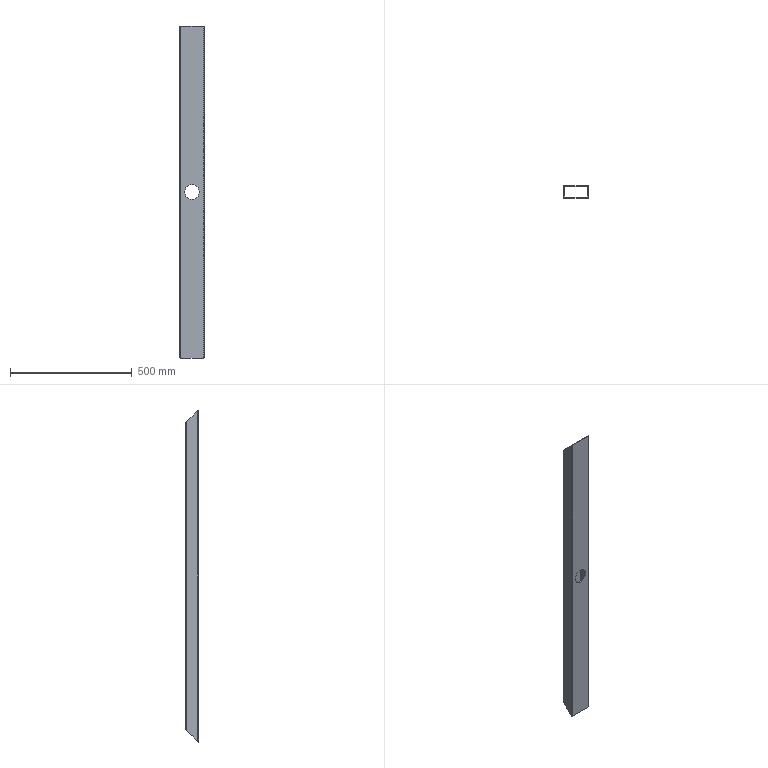Part | SolidWorks | features ICE 2, Extrusion 1 | 1 solid | 22 faces | box 100 x 50 x 1364 mm | volume 1106656 mm3 | cylinder 12 | plane 10 | commonest cylinder face diameters 0.4 x4 6.4 x4 60.3 x4
STEP:
#1=CARTESIAN_POINT('',(0.,-25.,656.26));
#2=VERTEX_POINT('',#1);
#3=CARTESIAN_POINT('',(0.,-25.,716.56));
#4=VERTEX_POINT('',#3);
#5=CARTESIAN_POINT('',(0.,-25.,686.41));
#6=DIRECTION('',(0.,1.,0.));
#7=DIRECTION('',(0.,0.,1.));
#8=AXIS2_PLACEMENT_3D('',#5,#6,#7);
#9=CIRCLE('',#8,30.15);
#10=EDGE_CURVE('',#2,#4,#9,.T.);
#11=ORIENTED_EDGE('',*,*,#10,.F.);
#12=CARTESIAN_POINT('',(0.,-22.,656.26));
#13=VERTEX_POINT('',#12);
#14=CARTESIAN_POINT('',(0.,-193.,656.26));
#15=DIRECTION('',(0.,1.,0.));
#16=VECTOR('',#15,1000.);
#17=LINE('',#14,#16);
#18=EDGE_CURVE('',#2,#13,#17,.T.);
#19=ORIENTED_EDGE('',*,*,#18,.T.);
#20=CARTESIAN_POINT('',(0.,-22.,716.56));
#21=VERTEX_POINT('',#20);
#22=CARTESIAN_POINT('',(0.,-22.,686.41));
#23=DIRECTION('',(0.,1.,0.));
#24=DIRECTION('',(0.,0.,1.));
#25=AXIS2_PLACEMENT_3D('',#22,#23,#24);
#26=CIRCLE('',#25,30.15);
#27=EDGE_CURVE('',#13,#21,#26,.T.);
#28=ORIENTED_EDGE('',*,*,#27,.T.);
#29=CARTESIAN_POINT('',(0.,-193.,716.56));
#30=DIRECTION('',(0.,1.,0.));
#31=VECTOR('',#30,1000.);
#32=LINE('',#29,#31);
#33=EDGE_CURVE('',#4,#21,#32,.T.);
#34=ORIENTED_EDGE('',*,*,#33,.F.);
#35=EDGE_LOOP('',(#11,#19,#28,#34));
#36=FACE_OUTER_BOUND('',#35,.T.);
#37=CARTESIAN_POINT('',(0.,-193.,686.41));
#38=DIRECTION('',(0.,1.,0.));
#39=DIRECTION('',(0.,0.,1.));
#40=AXIS2_PLACEMENT_3D('',#37,#38,#39);
#41=CYLINDRICAL_SURFACE('',#40,30.15);
#42=ADVANCED_FACE('',(#36),#41,.F.);
#43=CARTESIAN_POINT('',(0.,22.,716.56));
#44=VERTEX_POINT('',#43);
#45=CARTESIAN_POINT('',(0.,22.,656.26));
#46=VERTEX_POINT('',#45);
#47=CARTESIAN_POINT('',(0.,22.,686.41));
#48=DIRECTION('',(0.,-1.,0.));
#49=DIRECTION('',(0.,0.,-1.));
#50=AXIS2_PLACEMENT_3D('',#47,#48,#49);
#51=CIRCLE('',#50,30.15);
#52=EDGE_CURVE('',#44,#46,#51,.T.);
#53=ORIENTED_EDGE('',*,*,#52,.T.);
#54=CARTESIAN_POINT('',(0.,25.,656.26));
#55=VERTEX_POINT('',#54);
#56=CARTESIAN_POINT('',(0.,-193.,656.26));
#57=DIRECTION('',(0.,1.,0.));
#58=VECTOR('',#57,1000.);
#59=LINE('',#56,#58);
#60=EDGE_CURVE('',#46,#55,#59,.T.);
#61=ORIENTED_EDGE('',*,*,#60,.T.);
#62=CARTESIAN_POINT('',(0.,25.,716.56));
#63=VERTEX_POINT('',#62);
#64=CARTESIAN_POINT('',(0.,25.,686.41));
#65=DIRECTION('',(0.,1.,0.));
#66=DIRECTION('',(0.,0.,1.));
#67=AXIS2_PLACEMENT_3D('',#64,#65,#66);
#68=CIRCLE('',#67,30.15);
#69=EDGE_CURVE('',#55,#63,#68,.T.);
#70=ORIENTED_EDGE('',*,*,#69,.T.);
#71=CARTESIAN_POINT('',(0.,-193.,716.56));
#72=DIRECTION('',(0.,1.,0.));
#73=VECTOR('',#72,1000.);
#74=LINE('',#71,#73);
#75=EDGE_CURVE('',#44,#63,#74,.T.);
#76=ORIENTED_EDGE('',*,*,#75,.F.);
#77=EDGE_LOOP('',(#53,#61,#70,#76));
#78=FACE_OUTER_BOUND('',#77,.T.);
#79=CARTESIAN_POINT('',(0.,-193.,686.41));
#80=DIRECTION('',(0.,1.,0.));
#81=DIRECTION('',(0.,0.,1.));
#82=AXIS2_PLACEMENT_3D('',#79,#80,#81);
#83=CYLINDRICAL_SURFACE('',#82,30.15);
#84=ADVANCED_FACE('',(#78),#83,.F.);
#85=ORIENTED_EDGE('',*,*,#52,.F.);
#86=CARTESIAN_POINT('',(0.,22.,686.41));
#87=DIRECTION('',(0.,-1.,0.));
#88=DIRECTION('',(0.,0.,-1.));
#89=AXIS2_PLACEMENT_3D('',#86,#87,#88);
#90=CIRCLE('',#89,30.15);
#91=EDGE_CURVE('',#46,#44,#90,.T.);
#92=ORIENTED_EDGE('',*,*,#91,.F.);
#93=EDGE_LOOP('',(#85,#92));
#94=FACE_BOUND('',#93,.T.);
#95=CARTESIAN_POINT('',(-46.8,22.,1321.41));
#96=VERTEX_POINT('',#95);
#97=CARTESIAN_POINT('',(46.8,22.,1321.41));
#98=VERTEX_POINT('',#97);
#99=CARTESIAN_POINT('',(-46.8,22.,1321.41));
#100=DIRECTION('',(1.,0.,0.));
#101=VECTOR('',#100,1000.);
#102=LINE('',#99,#101);
#103=EDGE_CURVE('',#96,#98,#102,.T.);
#104=ORIENTED_EDGE('',*,*,#103,.F.);
#105=CARTESIAN_POINT('',(-46.8,22.,51.41));
#106=VERTEX_POINT('',#105);
#107=CARTESIAN_POINT('',(-46.8,22.,1400.));
#108=DIRECTION('',(0.,0.,-1.));
#109=VECTOR('',#108,1000.);
#110=LINE('',#107,#109);
#111=EDGE_CURVE('',#96,#106,#110,.T.);
#112=ORIENTED_EDGE('',*,*,#111,.T.);
#113=CARTESIAN_POINT('',(46.8,22.,51.41));
#114=VERTEX_POINT('',#113);
#115=CARTESIAN_POINT('',(-46.8,22.,51.41));
#116=DIRECTION('',(-1.,0.,0.));
#117=VECTOR('',#116,1000.);
#118=LINE('',#115,#117);
#119=EDGE_CURVE('',#114,#106,#118,.T.);
#120=ORIENTED_EDGE('',*,*,#119,.F.);
#121=CARTESIAN_POINT('',(46.8,22.,1400.));
#122=DIRECTION('',(0.,0.,-1.));
#123=VECTOR('',#122,1000.);
#124=LINE('',#121,#123);
#125=EDGE_CURVE('',#98,#114,#124,.T.);
#126=ORIENTED_EDGE('',*,*,#125,.F.);
#127=EDGE_LOOP('',(#104,#112,#120,#126));
#128=FACE_OUTER_BOUND('',#127,.T.);
#129=CARTESIAN_POINT('',(-46.8,22.,1400.));
#130=DIRECTION('',(0.,-1.,0.));
#131=DIRECTION('',(0.,0.,-1.));
#132=AXIS2_PLACEMENT_3D('',#129,#130,#131);
#133=PLANE('',#132);
#134=ADVANCED_FACE('',(#94,#128),#133,.T.);
#135=CARTESIAN_POINT('',(47.,21.8,1321.61));
#136=VERTEX_POINT('',#135);
#137=CARTESIAN_POINT('',(46.8,22.,1321.41));
#138=CARTESIAN_POINT('',(46.917,22.,1321.41));
#139=CARTESIAN_POINT('',(47.,21.917,1321.493));
#140=CARTESIAN_POINT('',(47.,21.8,1321.61));
#141=(BOUNDED_CURVE()B_SPLINE_CURVE(3,(#137,#138,#139,#140),.UNSPECIFIED.,.F.,.F.)B_SPLINE_CURVE_WITH_KNOTS((4,4),(0.,1.571),.UNSPECIFIED.)CURVE()GEOMETRIC_REPRESENTATION_ITEM()RATIONAL_B_SPLINE_CURVE((1.,0.8047,0.8047,1.))REPRESENTATION_ITEM(''));
#142=EDGE_CURVE('',#98,#136,#141,.T.);
#143=ORIENTED_EDGE('',*,*,#142,.F.);
#144=ORIENTED_EDGE('',*,*,#125,.T.);
#145=CARTESIAN_POINT('',(47.,21.8,51.21));
#146=VERTEX_POINT('',#145);
#147=CARTESIAN_POINT('',(47.,21.8,51.21));
#148=CARTESIAN_POINT('',(47.,21.917,51.327));
#149=CARTESIAN_POINT('',(46.917,22.,51.41));
#150=CARTESIAN_POINT('',(46.8,22.,51.41));
#151=(BOUNDED_CURVE()B_SPLINE_CURVE(3,(#147,#148,#149,#150),.UNSPECIFIED.,.F.,.F.)B_SPLINE_CURVE_WITH_KNOTS((4,4),(1.571,3.142),.UNSPECIFIED.)CURVE()GEOMETRIC_REPRESENTATION_ITEM()RATIONAL_B_SPLINE_CURVE((1.,0.8047,0.8047,1.))REPRESENTATION_ITEM(''));
#152=EDGE_CURVE('',#146,#114,#151,.T.);
#153=ORIENTED_EDGE('',*,*,#152,.F.);
#154=CARTESIAN_POINT('',(47.,21.8,1400.));
#155=DIRECTION('',(0.,0.,-1.));
#156=VECTOR('',#155,1000.);
#157=LINE('',#154,#156);
#158=EDGE_CURVE('',#136,#146,#157,.T.);
#159=ORIENTED_EDGE('',*,*,#158,.F.);
#160=EDGE_LOOP('',(#143,#144,#153,#159));
#161=FACE_OUTER_BOUND('',#160,.T.);
#162=CARTESIAN_POINT('',(46.8,21.8,1400.));
#163=DIRECTION('',(0.,0.,-1.));
#164=DIRECTION('',(-1.,0.,0.));
#165=AXIS2_PLACEMENT_3D('',#162,#163,#164);
#166=CYLINDRICAL_SURFACE('',#165,0.2);
#167=ADVANCED_FACE('',(#161),#166,.F.);
#168=CARTESIAN_POINT('',(47.,-21.8,1365.21));
#169=VERTEX_POINT('',#168);
#170=CARTESIAN_POINT('',(47.,-17.395,1360.805));
#171=DIRECTION('',(0.,-0.7071,0.7071));
#172=VECTOR('',#171,1000.);
#173=LINE('',#170,#172);
#174=EDGE_CURVE('',#136,#169,#173,.T.);
#175=ORIENTED_EDGE('',*,*,#174,.F.);
#176=ORIENTED_EDGE('',*,*,#158,.T.);
#177=CARTESIAN_POINT('',(47.,-21.8,7.61));
#178=VERTEX_POINT('',#177);
#179=CARTESIAN_POINT('',(47.,696.195,725.605));
#180=DIRECTION('',(0.,0.7071,0.7071));
#181=VECTOR('',#180,1000.);
#182=LINE('',#179,#181);
#183=EDGE_CURVE('',#178,#146,#182,.T.);
#184=ORIENTED_EDGE('',*,*,#183,.F.);
#185=CARTESIAN_POINT('',(47.,-21.8,1400.));
#186=DIRECTION('',(0.,0.,-1.));
#187=VECTOR('',#186,1000.);
#188=LINE('',#185,#187);
#189=EDGE_CURVE('',#169,#178,#188,.T.);
#190=ORIENTED_EDGE('',*,*,#189,.F.);
#191=EDGE_LOOP('',(#175,#176,#184,#190));
#192=FACE_OUTER_BOUND('',#191,.T.);
#193=CARTESIAN_POINT('',(47.,21.8,1400.));
#194=DIRECTION('',(-1.,0.,0.));
#195=DIRECTION('',(0.,0.,1.));
#196=AXIS2_PLACEMENT_3D('',#193,#194,#195);
#197=PLANE('',#196);
#198=ADVANCED_FACE('',(#192),#197,.T.);
#199=CARTESIAN_POINT('',(46.8,-22.,1365.41));
#200=VERTEX_POINT('',#199);
#201=CARTESIAN_POINT('',(47.,-21.8,1365.21));
#202=CARTESIAN_POINT('',(47.,-21.917,1365.327));
#203=CARTESIAN_POINT('',(46.917,-22.,1365.41));
#204=CARTESIAN_POINT('',(46.8,-22.,1365.41));
#205=(BOUNDED_CURVE()B_SPLINE_CURVE(3,(#201,#202,#203,#204),.UNSPECIFIED.,.F.,.F.)B_SPLINE_CURVE_WITH_KNOTS((4,4),(1.571,3.142),.UNSPECIFIED.)CURVE()GEOMETRIC_REPRESENTATION_ITEM()RATIONAL_B_SPLINE_CURVE((1.,0.8047,0.8047,1.))REPRESENTATION_ITEM(''));
#206=EDGE_CURVE('',#169,#200,#205,.T.);
#207=ORIENTED_EDGE('',*,*,#206,.F.);
#208=ORIENTED_EDGE('',*,*,#189,.T.);
#209=CARTESIAN_POINT('',(46.8,-22.,7.41));
#210=VERTEX_POINT('',#209);
#211=CARTESIAN_POINT('',(46.8,-22.,7.41));
#212=CARTESIAN_POINT('',(46.917,-22.,7.41));
#213=CARTESIAN_POINT('',(47.,-21.917,7.493));
#214=CARTESIAN_POINT('',(47.,-21.8,7.61));
#215=(BOUNDED_CURVE()B_SPLINE_CURVE(3,(#211,#212,#213,#214),.UNSPECIFIED.,.F.,.F.)B_SPLINE_CURVE_WITH_KNOTS((4,4),(0.,1.571),.UNSPECIFIED.)CURVE()GEOMETRIC_REPRESENTATION_ITEM()RATIONAL_B_SPLINE_CURVE((1.,0.8047,0.8047,1.))REPRESENTATION_ITEM(''));
#216=EDGE_CURVE('',#210,#178,#215,.T.);
#217=ORIENTED_EDGE('',*,*,#216,.F.);
#218=CARTESIAN_POINT('',(46.8,-22.,1400.));
#219=DIRECTION('',(0.,0.,-1.));
#220=VECTOR('',#219,1000.);
#221=LINE('',#218,#220);
#222=EDGE_CURVE('',#200,#210,#221,.T.);
#223=ORIENTED_EDGE('',*,*,#222,.F.);
#224=EDGE_LOOP('',(#207,#208,#217,#223));
#225=FACE_OUTER_BOUND('',#224,.T.);
#226=CARTESIAN_POINT('',(46.8,-21.8,1400.));
#227=DIRECTION('',(0.,0.,-1.));
#228=DIRECTION('',(-1.,0.,0.));
#229=AXIS2_PLACEMENT_3D('',#226,#227,#228);
#230=CYLINDRICAL_SURFACE('',#229,0.2);
#231=ADVANCED_FACE('',(#225),#230,.F.);
#232=CARTESIAN_POINT('',(0.,-22.,686.41));
#233=DIRECTION('',(0.,1.,0.));
#234=DIRECTION('',(0.,0.,1.));
#235=AXIS2_PLACEMENT_3D('',#232,#233,#234);
#236=CIRCLE('',#235,30.15);
#237=EDGE_CURVE('',#21,#13,#236,.T.);
#238=ORIENTED_EDGE('',*,*,#237,.F.);
#239=ORIENTED_EDGE('',*,*,#27,.F.);
#240=EDGE_LOOP('',(#238,#239));
#241=FACE_BOUND('',#240,.T.);
#242=CARTESIAN_POINT('',(-46.8,-22.,1365.41));
#243=VERTEX_POINT('',#242);
#244=CARTESIAN_POINT('',(-46.8,-22.,1365.41));
#245=DIRECTION('',(-1.,0.,0.));
#246=VECTOR('',#245,1000.);
#247=LINE('',#244,#246);
#248=EDGE_CURVE('',#200,#243,#247,.T.);
#249=ORIENTED_EDGE('',*,*,#248,.F.);
#250=ORIENTED_EDGE('',*,*,#222,.T.);
#251=CARTESIAN_POINT('',(-46.8,-22.,7.41));
#252=VERTEX_POINT('',#251);
#253=CARTESIAN_POINT('',(-46.8,-22.,7.41));
#254=DIRECTION('',(1.,0.,0.));
#255=VECTOR('',#254,1000.);
#256=LINE('',#253,#255);
#257=EDGE_CURVE('',#252,#210,#256,.T.);
#258=ORIENTED_EDGE('',*,*,#257,.F.);
#259=CARTESIAN_POINT('',(-46.8,-22.,1400.));
#260=DIRECTION('',(0.,0.,-1.));
#261=VECTOR('',#260,1000.);
#262=LINE('',#259,#261);
#263=EDGE_CURVE('',#243,#252,#262,.T.);
#264=ORIENTED_EDGE('',*,*,#263,.F.);
#265=EDGE_LOOP('',(#249,#250,#258,#264));
#266=FACE_OUTER_BOUND('',#265,.T.);
#267=CARTESIAN_POINT('',(-46.8,-22.,1400.));
#268=DIRECTION('',(0.,1.,0.));
#269=DIRECTION('',(0.,0.,1.));
#270=AXIS2_PLACEMENT_3D('',#267,#268,#269);
#271=PLANE('',#270);
#272=ADVANCED_FACE('',(#241,#266),#271,.T.);
#273=CARTESIAN_POINT('',(-47.,-21.8,1365.21));
#274=VERTEX_POINT('',#273);
#275=CARTESIAN_POINT('',(-46.8,-22.,1365.41));
#276=CARTESIAN_POINT('',(-46.917,-22.,1365.41));
#277=CARTESIAN_POINT('',(-47.,-21.917,1365.327));
#278=CARTESIAN_POINT('',(-47.,-21.8,1365.21));
#279=(BOUNDED_CURVE()B_SPLINE_CURVE(3,(#275,#276,#277,#278),.UNSPECIFIED.,.F.,.F.)B_SPLINE_CURVE_WITH_KNOTS((4,4),(3.142,4.712),.UNSPECIFIED.)CURVE()GEOMETRIC_REPRESENTATION_ITEM()RATIONAL_B_SPLINE_CURVE((1.,0.8047,0.8047,1.))REPRESENTATION_ITEM(''));
#280=EDGE_CURVE('',#243,#274,#279,.T.);
#281=ORIENTED_EDGE('',*,*,#280,.F.);
#282=ORIENTED_EDGE('',*,*,#263,.T.);
#283=CARTESIAN_POINT('',(-47.,-21.8,7.61));
#284=VERTEX_POINT('',#283);
#285=CARTESIAN_POINT('',(-47.,-21.8,7.61));
#286=CARTESIAN_POINT('',(-47.,-21.917,7.493));
#287=CARTESIAN_POINT('',(-46.917,-22.,7.41));
#288=CARTESIAN_POINT('',(-46.8,-22.,7.41));
#289=(BOUNDED_CURVE()B_SPLINE_CURVE(3,(#285,#286,#287,#288),.UNSPECIFIED.,.F.,.T.)B_SPLINE_CURVE_WITH_KNOTS((4,4),(4.712,6.283),.UNSPECIFIED.)CURVE()GEOMETRIC_REPRESENTATION_ITEM()RATIONAL_B_SPLINE_CURVE((1.,0.8047,0.8047,1.))REPRESENTATION_ITEM(''));
#290=EDGE_CURVE('',#284,#252,#289,.T.);
#291=ORIENTED_EDGE('',*,*,#290,.F.);
#292=CARTESIAN_POINT('',(-47.,-21.8,1400.));
#293=DIRECTION('',(0.,0.,-1.));
#294=VECTOR('',#293,1000.);
#295=LINE('',#292,#294);
#296=EDGE_CURVE('',#274,#284,#295,.T.);
#297=ORIENTED_EDGE('',*,*,#296,.F.);
#298=EDGE_LOOP('',(#281,#282,#291,#297));
#299=FACE_OUTER_BOUND('',#298,.T.);
#300=CARTESIAN_POINT('',(-46.8,-21.8,1400.));
#301=DIRECTION('',(0.,0.,-1.));
#302=DIRECTION('',(-1.,0.,0.));
#303=AXIS2_PLACEMENT_3D('',#300,#301,#302);
#304=CYLINDRICAL_SURFACE('',#303,0.2);
#305=ADVANCED_FACE('',(#299),#304,.F.);
#306=CARTESIAN_POINT('',(-47.,21.8,1321.61));
#307=VERTEX_POINT('',#306);
#308=CARTESIAN_POINT('',(-47.,-17.395,1360.805));
#309=DIRECTION('',(0.,0.7071,-0.7071));
#310=VECTOR('',#309,1000.);
#311=LINE('',#308,#310);
#312=EDGE_CURVE('',#274,#307,#311,.T.);
#313=ORIENTED_EDGE('',*,*,#312,.F.);
#314=ORIENTED_EDGE('',*,*,#296,.T.);
#315=CARTESIAN_POINT('',(-47.,21.8,51.21));
#316=VERTEX_POINT('',#315);
#317=CARTESIAN_POINT('',(-47.,696.195,725.605));
#318=DIRECTION('',(0.,-0.7071,-0.7071));
#319=VECTOR('',#318,1000.);
#320=LINE('',#317,#319);
#321=EDGE_CURVE('',#316,#284,#320,.T.);
#322=ORIENTED_EDGE('',*,*,#321,.F.);
#323=CARTESIAN_POINT('',(-47.,21.8,1400.));
#324=DIRECTION('',(0.,0.,-1.));
#325=VECTOR('',#324,1000.);
#326=LINE('',#323,#325);
#327=EDGE_CURVE('',#307,#316,#326,.T.);
#328=ORIENTED_EDGE('',*,*,#327,.F.);
#329=EDGE_LOOP('',(#313,#314,#322,#328));
#330=FACE_OUTER_BOUND('',#329,.T.);
#331=CARTESIAN_POINT('',(-47.,21.8,1400.));
#332=DIRECTION('',(1.,0.,0.));
#333=DIRECTION('',(0.,0.,-1.));
#334=AXIS2_PLACEMENT_3D('',#331,#332,#333);
#335=PLANE('',#334);
#336=ADVANCED_FACE('',(#330),#335,.T.);
#337=CARTESIAN_POINT('',(-47.,21.8,1321.61));
#338=CARTESIAN_POINT('',(-47.,21.917,1321.493));
#339=CARTESIAN_POINT('',(-46.917,22.,1321.41));
#340=CARTESIAN_POINT('',(-46.8,22.,1321.41));
#341=(BOUNDED_CURVE()B_SPLINE_CURVE(3,(#337,#338,#339,#340),.UNSPECIFIED.,.F.,.F.)B_SPLINE_CURVE_WITH_KNOTS((4,4),(4.712,6.283),.UNSPECIFIED.)CURVE()GEOMETRIC_REPRESENTATION_ITEM()RATIONAL_B_SPLINE_CURVE((1.,0.8047,0.8047,1.))REPRESENTATION_ITEM(''));
#342=EDGE_CURVE('',#307,#96,#341,.T.);
#343=ORIENTED_EDGE('',*,*,#342,.F.);
#344=ORIENTED_EDGE('',*,*,#327,.T.);
#345=CARTESIAN_POINT('',(-46.8,22.,51.41));
#346=CARTESIAN_POINT('',(-46.917,22.,51.41));
#347=CARTESIAN_POINT('',(-47.,21.917,51.327));
#348=CARTESIAN_POINT('',(-47.,21.8,51.21));
#349=(BOUNDED_CURVE()B_SPLINE_CURVE(3,(#345,#346,#347,#348),.UNSPECIFIED.,.F.,.F.)B_SPLINE_CURVE_WITH_KNOTS((4,4),(3.142,4.712),.UNSPECIFIED.)CURVE()GEOMETRIC_REPRESENTATION_ITEM()RATIONAL_B_SPLINE_CURVE((1.,0.8047,0.8047,1.))REPRESENTATION_ITEM(''));
#350=EDGE_CURVE('',#106,#316,#349,.T.);
#351=ORIENTED_EDGE('',*,*,#350,.F.);
#352=ORIENTED_EDGE('',*,*,#111,.F.);
#353=EDGE_LOOP('',(#343,#344,#351,#352));
#354=FACE_OUTER_BOUND('',#353,.T.);
#355=CARTESIAN_POINT('',(-46.8,21.8,1400.));
#356=DIRECTION('',(0.,0.,-1.));
#357=DIRECTION('',(-1.,0.,0.));
#358=AXIS2_PLACEMENT_3D('',#355,#356,#357);
#359=CYLINDRICAL_SURFACE('',#358,0.2);
#360=ADVANCED_FACE('',(#354),#359,.F.);
#361=ORIENTED_EDGE('',*,*,#350,.T.);
#362=ORIENTED_EDGE('',*,*,#321,.T.);
#363=ORIENTED_EDGE('',*,*,#290,.T.);
#364=ORIENTED_EDGE('',*,*,#257,.T.);
#365=ORIENTED_EDGE('',*,*,#216,.T.);
#366=ORIENTED_EDGE('',*,*,#183,.T.);
#367=ORIENTED_EDGE('',*,*,#152,.T.);
#368=ORIENTED_EDGE('',*,*,#119,.T.);
#369=EDGE_LOOP('',(#361,#362,#363,#364,#365,#366,#367,#368));
#370=FACE_BOUND('',#369,.T.);
#371=CARTESIAN_POINT('',(-46.8,-25.,4.41));
#372=VERTEX_POINT('',#371);
#373=CARTESIAN_POINT('',(46.8,-25.,4.41));
#374=VERTEX_POINT('',#373);
#375=CARTESIAN_POINT('',(-1350.,-25.,4.41));
#376=DIRECTION('',(1.,0.,0.));
#377=VECTOR('',#376,1000.);
#378=LINE('',#375,#377);
#379=EDGE_CURVE('',#372,#374,#378,.T.);
#380=ORIENTED_EDGE('',*,*,#379,.F.);
#381=CARTESIAN_POINT('',(-50.,-21.8,7.61));
#382=VERTEX_POINT('',#381);
#383=CARTESIAN_POINT('',(-50.,-21.8,7.61));
#384=CARTESIAN_POINT('',(-50.,-23.675,5.736));
#385=CARTESIAN_POINT('',(-48.675,-25.,4.41));
#386=CARTESIAN_POINT('',(-46.8,-25.,4.41));
#387=(BOUNDED_CURVE()B_SPLINE_CURVE(3,(#383,#384,#385,#386),.UNSPECIFIED.,.F.,.F.)B_SPLINE_CURVE_WITH_KNOTS((4,4),(4.712,6.283),.UNSPECIFIED.)CURVE()GEOMETRIC_REPRESENTATION_ITEM()RATIONAL_B_SPLINE_CURVE((1.,0.8047,0.8047,1.))REPRESENTATION_ITEM(''));
#388=EDGE_CURVE('',#382,#372,#387,.T.);
#389=ORIENTED_EDGE('',*,*,#388,.F.);
#390=CARTESIAN_POINT('',(-50.,21.8,51.21));
#391=VERTEX_POINT('',#390);
#392=CARTESIAN_POINT('',(-50.,696.195,725.605));
#393=DIRECTION('',(0.,-0.7071,-0.7071));
#394=VECTOR('',#393,1000.);
#395=LINE('',#392,#394);
#396=EDGE_CURVE('',#391,#382,#395,.T.);
#397=ORIENTED_EDGE('',*,*,#396,.F.);
#398=CARTESIAN_POINT('',(-46.8,25.,54.41));
#399=VERTEX_POINT('',#398);
#400=CARTESIAN_POINT('',(-46.8,25.,54.41));
#401=CARTESIAN_POINT('',(-48.675,25.,54.41));
#402=CARTESIAN_POINT('',(-50.,23.675,53.085));
#403=CARTESIAN_POINT('',(-50.,21.8,51.21));
#404=(BOUNDED_CURVE()B_SPLINE_CURVE(3,(#400,#401,#402,#403),.UNSPECIFIED.,.F.,.F.)B_SPLINE_CURVE_WITH_KNOTS((4,4),(3.142,4.712),.UNSPECIFIED.)CURVE()GEOMETRIC_REPRESENTATION_ITEM()RATIONAL_B_SPLINE_CURVE((1.,0.8047,0.8047,1.))REPRESENTATION_ITEM(''));
#405=EDGE_CURVE('',#399,#391,#404,.T.);
#406=ORIENTED_EDGE('',*,*,#405,.F.);
#407=CARTESIAN_POINT('',(46.8,25.,54.41));
#408=VERTEX_POINT('',#407);
#409=CARTESIAN_POINT('',(-1350.,25.,54.41));
#410=DIRECTION('',(1.,0.,0.));
#411=VECTOR('',#410,1000.);
#412=LINE('',#409,#411);
#413=EDGE_CURVE('',#399,#408,#412,.T.);
#414=ORIENTED_EDGE('',*,*,#413,.T.);
#415=CARTESIAN_POINT('',(50.,21.8,51.21));
#416=VERTEX_POINT('',#415);
#417=CARTESIAN_POINT('',(50.,21.8,51.21));
#418=CARTESIAN_POINT('',(50.,23.675,53.085));
#419=CARTESIAN_POINT('',(48.675,25.,54.41));
#420=CARTESIAN_POINT('',(46.8,25.,54.41));
#421=(BOUNDED_CURVE()B_SPLINE_CURVE(3,(#417,#418,#419,#420),.UNSPECIFIED.,.F.,.F.)B_SPLINE_CURVE_WITH_KNOTS((4,4),(1.571,3.142),.UNSPECIFIED.)CURVE()GEOMETRIC_REPRESENTATION_ITEM()RATIONAL_B_SPLINE_CURVE((1.,0.8047,0.8047,1.))REPRESENTATION_ITEM(''));
#422=EDGE_CURVE('',#416,#408,#421,.T.);
#423=ORIENTED_EDGE('',*,*,#422,.F.);
#424=CARTESIAN_POINT('',(50.,-21.8,7.61));
#425=VERTEX_POINT('',#424);
#426=CARTESIAN_POINT('',(50.,25.,54.41));
#427=DIRECTION('',(0.,-0.7071,-0.7071));
#428=VECTOR('',#427,1000.);
#429=LINE('',#426,#428);
#430=EDGE_CURVE('',#416,#425,#429,.T.);
#431=ORIENTED_EDGE('',*,*,#430,.T.);
#432=CARTESIAN_POINT('',(46.8,-25.,4.41));
#433=CARTESIAN_POINT('',(48.675,-25.,4.41));
#434=CARTESIAN_POINT('',(50.,-23.675,5.736));
#435=CARTESIAN_POINT('',(50.,-21.8,7.61));
#436=(BOUNDED_CURVE()B_SPLINE_CURVE(3,(#432,#433,#434,#435),.UNSPECIFIED.,.F.,.F.)B_SPLINE_CURVE_WITH_KNOTS((4,4),(0.,1.571),.UNSPECIFIED.)CURVE()GEOMETRIC_REPRESENTATION_ITEM()RATIONAL_B_SPLINE_CURVE((1.,0.8047,0.8047,1.))REPRESENTATION_ITEM(''));
#437=EDGE_CURVE('',#374,#425,#436,.T.);
#438=ORIENTED_EDGE('',*,*,#437,.F.);
#439=EDGE_LOOP('',(#380,#389,#397,#406,#414,#423,#431,#438));
#440=FACE_OUTER_BOUND('',#439,.T.);
#441=CARTESIAN_POINT('',(-1350.,25.,54.41));
#442=DIRECTION('',(0.,-0.7071,0.7071));
#443=DIRECTION('',(0.,-0.7071,-0.7071));
#444=AXIS2_PLACEMENT_3D('',#441,#442,#443);
#445=PLANE('',#444);
#446=ADVANCED_FACE('',(#370,#440),#445,.F.);
#447=ORIENTED_EDGE('',*,*,#342,.T.);
#448=ORIENTED_EDGE('',*,*,#103,.T.);
#449=ORIENTED_EDGE('',*,*,#142,.T.);
#450=ORIENTED_EDGE('',*,*,#174,.T.);
#451=ORIENTED_EDGE('',*,*,#206,.T.);
#452=ORIENTED_EDGE('',*,*,#248,.T.);
#453=ORIENTED_EDGE('',*,*,#280,.T.);
#454=ORIENTED_EDGE('',*,*,#312,.T.);
#455=EDGE_LOOP('',(#447,#448,#449,#450,#451,#452,#453,#454));
#456=FACE_BOUND('',#455,.T.);
#457=CARTESIAN_POINT('',(50.,-21.8,1365.21));
#458=VERTEX_POINT('',#457);
#459=CARTESIAN_POINT('',(50.,21.8,1321.61));
#460=VERTEX_POINT('',#459);
#461=CARTESIAN_POINT('',(50.,25.,1318.41));
#462=DIRECTION('',(0.,0.7071,-0.7071));
#463=VECTOR('',#462,1000.);
#464=LINE('',#461,#463);
#465=EDGE_CURVE('',#458,#460,#464,.T.);
#466=ORIENTED_EDGE('',*,*,#465,.T.);
#467=CARTESIAN_POINT('',(46.8,25.,1318.41));
#468=VERTEX_POINT('',#467);
#469=CARTESIAN_POINT('',(46.8,25.,1318.41));
#470=CARTESIAN_POINT('',(48.675,25.,1318.41));
#471=CARTESIAN_POINT('',(50.,23.675,1319.736));
#472=CARTESIAN_POINT('',(50.,21.8,1321.61));
#473=(BOUNDED_CURVE()B_SPLINE_CURVE(3,(#469,#470,#471,#472),.UNSPECIFIED.,.F.,.F.)B_SPLINE_CURVE_WITH_KNOTS((4,4),(0.,1.571),.UNSPECIFIED.)CURVE()GEOMETRIC_REPRESENTATION_ITEM()RATIONAL_B_SPLINE_CURVE((1.,0.8047,0.8047,1.))REPRESENTATION_ITEM(''));
#474=EDGE_CURVE('',#468,#460,#473,.T.);
#475=ORIENTED_EDGE('',*,*,#474,.F.);
#476=CARTESIAN_POINT('',(-46.8,25.,1318.41));
#477=VERTEX_POINT('',#476);
#478=CARTESIAN_POINT('',(-1350.,25.,1318.41));
#479=DIRECTION('',(1.,0.,0.));
#480=VECTOR('',#479,1000.);
#481=LINE('',#478,#480);
#482=EDGE_CURVE('',#477,#468,#481,.T.);
#483=ORIENTED_EDGE('',*,*,#482,.F.);
#484=CARTESIAN_POINT('',(-50.,21.8,1321.61));
#485=VERTEX_POINT('',#484);
#486=CARTESIAN_POINT('',(-50.,21.8,1321.61));
#487=CARTESIAN_POINT('',(-50.,23.675,1319.736));
#488=CARTESIAN_POINT('',(-48.675,25.,1318.41));
#489=CARTESIAN_POINT('',(-46.8,25.,1318.41));
#490=(BOUNDED_CURVE()B_SPLINE_CURVE(3,(#486,#487,#488,#489),.UNSPECIFIED.,.F.,.T.)B_SPLINE_CURVE_WITH_KNOTS((4,4),(4.712,6.283),.UNSPECIFIED.)CURVE()GEOMETRIC_REPRESENTATION_ITEM()RATIONAL_B_SPLINE_CURVE((1.,0.8047,0.8047,1.))REPRESENTATION_ITEM(''));
#491=EDGE_CURVE('',#485,#477,#490,.T.);
#492=ORIENTED_EDGE('',*,*,#491,.F.);
#493=CARTESIAN_POINT('',(-50.,-21.8,1365.21));
#494=VERTEX_POINT('',#493);
#495=CARTESIAN_POINT('',(-50.,-17.395,1360.805));
#496=DIRECTION('',(0.,0.7071,-0.7071));
#497=VECTOR('',#496,1000.);
#498=LINE('',#495,#497);
#499=EDGE_CURVE('',#494,#485,#498,.T.);
#500=ORIENTED_EDGE('',*,*,#499,.F.);
#501=CARTESIAN_POINT('',(-46.8,-25.,1368.41));
#502=VERTEX_POINT('',#501);
#503=CARTESIAN_POINT('',(-46.8,-25.,1368.41));
#504=CARTESIAN_POINT('',(-48.675,-25.,1368.41));
#505=CARTESIAN_POINT('',(-50.,-23.675,1367.085));
#506=CARTESIAN_POINT('',(-50.,-21.8,1365.21));
#507=(BOUNDED_CURVE()B_SPLINE_CURVE(3,(#503,#504,#505,#506),.UNSPECIFIED.,.F.,.F.)B_SPLINE_CURVE_WITH_KNOTS((4,4),(3.142,4.712),.UNSPECIFIED.)CURVE()GEOMETRIC_REPRESENTATION_ITEM()RATIONAL_B_SPLINE_CURVE((1.,0.8047,0.8047,1.))REPRESENTATION_ITEM(''));
#508=EDGE_CURVE('',#502,#494,#507,.T.);
#509=ORIENTED_EDGE('',*,*,#508,.F.);
#510=CARTESIAN_POINT('',(46.8,-25.,1368.41));
#511=VERTEX_POINT('',#510);
#512=CARTESIAN_POINT('',(-1350.,-25.,1368.41));
#513=DIRECTION('',(1.,0.,0.));
#514=VECTOR('',#513,1000.);
#515=LINE('',#512,#514);
#516=EDGE_CURVE('',#502,#511,#515,.T.);
#517=ORIENTED_EDGE('',*,*,#516,.T.);
#518=CARTESIAN_POINT('',(50.,-21.8,1365.21));
#519=CARTESIAN_POINT('',(50.,-23.675,1367.085));
#520=CARTESIAN_POINT('',(48.675,-25.,1368.41));
#521=CARTESIAN_POINT('',(46.8,-25.,1368.41));
#522=(BOUNDED_CURVE()B_SPLINE_CURVE(3,(#518,#519,#520,#521),.UNSPECIFIED.,.F.,.F.)B_SPLINE_CURVE_WITH_KNOTS((4,4),(1.571,3.142),.UNSPECIFIED.)CURVE()GEOMETRIC_REPRESENTATION_ITEM()RATIONAL_B_SPLINE_CURVE((1.,0.8047,0.8047,1.))REPRESENTATION_ITEM(''));
#523=EDGE_CURVE('',#458,#511,#522,.T.);
#524=ORIENTED_EDGE('',*,*,#523,.F.);
#525=EDGE_LOOP('',(#466,#475,#483,#492,#500,#509,#517,#524));
#526=FACE_OUTER_BOUND('',#525,.T.);
#527=CARTESIAN_POINT('',(-1350.,25.,1318.41));
#528=DIRECTION('',(0.,-0.7071,-0.7071));
#529=DIRECTION('',(0.,0.7071,-0.7071));
#530=AXIS2_PLACEMENT_3D('',#527,#528,#529);
#531=PLANE('',#530);
#532=ADVANCED_FACE('',(#456,#526),#531,.F.);
#533=CARTESIAN_POINT('',(-46.8,-25.,1400.));
#534=DIRECTION('',(0.,0.,-1.));
#535=VECTOR('',#534,1000.);
#536=LINE('',#533,#535);
#537=EDGE_CURVE('',#502,#372,#536,.T.);
#538=ORIENTED_EDGE('',*,*,#537,.F.);
#539=ORIENTED_EDGE('',*,*,#508,.T.);
#540=CARTESIAN_POINT('',(-50.,-21.8,1400.));
#541=DIRECTION('',(0.,0.,-1.));
#542=VECTOR('',#541,1000.);
#543=LINE('',#540,#542);
#544=EDGE_CURVE('',#494,#382,#543,.T.);
#545=ORIENTED_EDGE('',*,*,#544,.T.);
#546=ORIENTED_EDGE('',*,*,#388,.T.);
#547=EDGE_LOOP('',(#538,#539,#545,#546));
#548=FACE_OUTER_BOUND('',#547,.T.);
#549=CARTESIAN_POINT('',(-46.8,-21.8,1400.));
#550=DIRECTION('',(0.,0.,-1.));
#551=DIRECTION('',(-1.,0.,0.));
#552=AXIS2_PLACEMENT_3D('',#549,#550,#551);
#553=CYLINDRICAL_SURFACE('',#552,3.2);
#554=ADVANCED_FACE('',(#548),#553,.T.);
#555=CARTESIAN_POINT('',(0.,-25.,686.41));
#556=DIRECTION('',(0.,1.,0.));
#557=DIRECTION('',(0.,0.,1.));
#558=AXIS2_PLACEMENT_3D('',#555,#556,#557);
#559=CIRCLE('',#558,30.15);
#560=EDGE_CURVE('',#4,#2,#559,.T.);
#561=ORIENTED_EDGE('',*,*,#560,.T.);
#562=ORIENTED_EDGE('',*,*,#10,.T.);
#563=EDGE_LOOP('',(#561,#562));
#564=FACE_BOUND('',#563,.T.);
#565=CARTESIAN_POINT('',(46.8,-25.,1400.));
#566=DIRECTION('',(0.,0.,-1.));
#567=VECTOR('',#566,1000.);
#568=LINE('',#565,#567);
#569=EDGE_CURVE('',#511,#374,#568,.T.);
#570=ORIENTED_EDGE('',*,*,#569,.F.);
#571=ORIENTED_EDGE('',*,*,#516,.F.);
#572=ORIENTED_EDGE('',*,*,#537,.T.);
#573=ORIENTED_EDGE('',*,*,#379,.T.);
#574=EDGE_LOOP('',(#570,#571,#572,#573));
#575=FACE_OUTER_BOUND('',#574,.T.);
#576=CARTESIAN_POINT('',(-46.8,-25.,1400.));
#577=DIRECTION('',(0.,1.,0.));
#578=DIRECTION('',(0.,0.,1.));
#579=AXIS2_PLACEMENT_3D('',#576,#577,#578);
#580=PLANE('',#579);
#581=ADVANCED_FACE('',(#564,#575),#580,.F.);
#582=CARTESIAN_POINT('',(50.,-21.8,1400.));
#583=DIRECTION('',(0.,0.,-1.));
#584=VECTOR('',#583,1000.);
#585=LINE('',#582,#584);
#586=EDGE_CURVE('',#458,#425,#585,.T.);
#587=ORIENTED_EDGE('',*,*,#586,.F.);
#588=ORIENTED_EDGE('',*,*,#523,.T.);
#589=ORIENTED_EDGE('',*,*,#569,.T.);
#590=ORIENTED_EDGE('',*,*,#437,.T.);
#591=EDGE_LOOP('',(#587,#588,#589,#590));
#592=FACE_OUTER_BOUND('',#591,.T.);
#593=CARTESIAN_POINT('',(46.8,-21.8,1400.));
#594=DIRECTION('',(0.,0.,-1.));
#595=DIRECTION('',(-1.,0.,0.));
#596=AXIS2_PLACEMENT_3D('',#593,#594,#595);
#597=CYLINDRICAL_SURFACE('',#596,3.2);
#598=ADVANCED_FACE('',(#592),#597,.T.);
#599=CARTESIAN_POINT('',(50.,21.8,1400.));
#600=DIRECTION('',(0.,0.,-1.));
#601=VECTOR('',#600,1000.);
#602=LINE('',#599,#601);
#603=EDGE_CURVE('',#460,#416,#602,.T.);
#604=ORIENTED_EDGE('',*,*,#603,.F.);
#605=ORIENTED_EDGE('',*,*,#465,.F.);
#606=ORIENTED_EDGE('',*,*,#586,.T.);
#607=ORIENTED_EDGE('',*,*,#430,.F.);
#608=EDGE_LOOP('',(#604,#605,#606,#607));
#609=FACE_OUTER_BOUND('',#608,.T.);
#610=CARTESIAN_POINT('',(50.,21.8,1400.));
#611=DIRECTION('',(-1.,0.,0.));
#612=DIRECTION('',(0.,-1.,0.));
#613=AXIS2_PLACEMENT_3D('',#610,#611,#612);
#614=PLANE('',#613);
#615=ADVANCED_FACE('',(#609),#614,.F.);
#616=CARTESIAN_POINT('',(46.8,25.,1400.));
#617=DIRECTION('',(0.,0.,-1.));
#618=VECTOR('',#617,1000.);
#619=LINE('',#616,#618);
#620=EDGE_CURVE('',#468,#408,#619,.T.);
#621=ORIENTED_EDGE('',*,*,#620,.F.);
#622=ORIENTED_EDGE('',*,*,#474,.T.);
#623=ORIENTED_EDGE('',*,*,#603,.T.);
#624=ORIENTED_EDGE('',*,*,#422,.T.);
#625=EDGE_LOOP('',(#621,#622,#623,#624));
#626=FACE_OUTER_BOUND('',#625,.T.);
#627=CARTESIAN_POINT('',(46.8,21.8,1400.));
#628=DIRECTION('',(0.,0.,-1.));
#629=DIRECTION('',(-1.,0.,0.));
#630=AXIS2_PLACEMENT_3D('',#627,#628,#629);
#631=CYLINDRICAL_SURFACE('',#630,3.2);
#632=ADVANCED_FACE('',(#626),#631,.T.);
#633=CARTESIAN_POINT('',(0.,25.,686.41));
#634=DIRECTION('',(0.,1.,0.));
#635=DIRECTION('',(0.,0.,1.));
#636=AXIS2_PLACEMENT_3D('',#633,#634,#635);
#637=CIRCLE('',#636,30.15);
#638=EDGE_CURVE('',#63,#55,#637,.T.);
#639=ORIENTED_EDGE('',*,*,#638,.F.);
#640=ORIENTED_EDGE('',*,*,#69,.F.);
#641=EDGE_LOOP('',(#639,#640));
#642=FACE_BOUND('',#641,.T.);
#643=CARTESIAN_POINT('',(-46.8,25.,1400.));
#644=DIRECTION('',(0.,0.,-1.));
#645=VECTOR('',#644,1000.);
#646=LINE('',#643,#645);
#647=EDGE_CURVE('',#477,#399,#646,.T.);
#648=ORIENTED_EDGE('',*,*,#647,.F.);
#649=ORIENTED_EDGE('',*,*,#482,.T.);
#650=ORIENTED_EDGE('',*,*,#620,.T.);
#651=ORIENTED_EDGE('',*,*,#413,.F.);
#652=EDGE_LOOP('',(#648,#649,#650,#651));
#653=FACE_OUTER_BOUND('',#652,.T.);
#654=CARTESIAN_POINT('',(-46.8,25.,1400.));
#655=DIRECTION('',(0.,-1.,0.));
#656=DIRECTION('',(0.,0.,-1.));
#657=AXIS2_PLACEMENT_3D('',#654,#655,#656);
#658=PLANE('',#657);
#659=ADVANCED_FACE('',(#642,#653),#658,.F.);
#660=CARTESIAN_POINT('',(-50.,21.8,1400.));
#661=DIRECTION('',(0.,0.,-1.));
#662=VECTOR('',#661,1000.);
#663=LINE('',#660,#662);
#664=EDGE_CURVE('',#485,#391,#663,.T.);
#665=ORIENTED_EDGE('',*,*,#664,.F.);
#666=ORIENTED_EDGE('',*,*,#491,.T.);
#667=ORIENTED_EDGE('',*,*,#647,.T.);
#668=ORIENTED_EDGE('',*,*,#405,.T.);
#669=EDGE_LOOP('',(#665,#666,#667,#668));
#670=FACE_OUTER_BOUND('',#669,.T.);
#671=CARTESIAN_POINT('',(-46.8,21.8,1400.));
#672=DIRECTION('',(0.,0.,-1.));
#673=DIRECTION('',(-1.,0.,0.));
#674=AXIS2_PLACEMENT_3D('',#671,#672,#673);
#675=CYLINDRICAL_SURFACE('',#674,3.2);
#676=ADVANCED_FACE('',(#670),#675,.T.);
#677=ORIENTED_EDGE('',*,*,#544,.F.);
#678=ORIENTED_EDGE('',*,*,#499,.T.);
#679=ORIENTED_EDGE('',*,*,#664,.T.);
#680=ORIENTED_EDGE('',*,*,#396,.T.);
#681=EDGE_LOOP('',(#677,#678,#679,#680));
#682=FACE_OUTER_BOUND('',#681,.T.);
#683=CARTESIAN_POINT('',(-50.,21.8,1400.));
#684=DIRECTION('',(1.,0.,0.));
#685=DIRECTION('',(0.,0.,-1.));
#686=AXIS2_PLACEMENT_3D('',#683,#684,#685);
#687=PLANE('',#686);
#688=ADVANCED_FACE('',(#682),#687,.F.);
#689=ORIENTED_EDGE('',*,*,#60,.F.);
#690=ORIENTED_EDGE('',*,*,#91,.T.);
#691=ORIENTED_EDGE('',*,*,#75,.T.);
#692=ORIENTED_EDGE('',*,*,#638,.T.);
#693=EDGE_LOOP('',(#689,#690,#691,#692));
#694=FACE_OUTER_BOUND('',#693,.T.);
#695=CARTESIAN_POINT('',(0.,-193.,686.41));
#696=DIRECTION('',(0.,1.,0.));
#697=DIRECTION('',(0.,0.,1.));
#698=AXIS2_PLACEMENT_3D('',#695,#696,#697);
#699=CYLINDRICAL_SURFACE('',#698,30.15);
#700=ADVANCED_FACE('',(#694),#699,.F.);
#701=ORIENTED_EDGE('',*,*,#18,.F.);
#702=ORIENTED_EDGE('',*,*,#560,.F.);
#703=ORIENTED_EDGE('',*,*,#33,.T.);
#704=ORIENTED_EDGE('',*,*,#237,.T.);
#705=EDGE_LOOP('',(#701,#702,#703,#704));
#706=FACE_OUTER_BOUND('',#705,.T.);
#707=CARTESIAN_POINT('',(0.,-193.,686.41));
#708=DIRECTION('',(0.,1.,0.));
#709=DIRECTION('',(0.,0.,1.));
#710=AXIS2_PLACEMENT_3D('',#707,#708,#709);
#711=CYLINDRICAL_SURFACE('',#710,30.15);
#712=ADVANCED_FACE('',(#706),#711,.F.);
#713=CLOSED_SHELL('',(#42,#84,#134,#167,#198,#231,#272,#305,#336,#360,#446,#532,#554,#581,#598,#615,#632,#659,#676,#688,#700,#712));
#714=MANIFOLD_SOLID_BREP('',#713);
#715=CARTESIAN_POINT('',(0.,0.,0.));
#716=DIRECTION('',(0.,0.,1.));
#717=DIRECTION('',(1.,0.,0.));
#718=AXIS2_PLACEMENT_3D('',#715,#716,#717);
#719=(LENGTH_UNIT()NAMED_UNIT(*)SI_UNIT(.MILLI.,.METRE.));
#720=UNCERTAINTY_MEASURE_WITH_UNIT(LENGTH_MEASURE(0.00001),#719,'','');
#721=(NAMED_UNIT(*)PLANE_ANGLE_UNIT()SI_UNIT($,.RADIAN.));
#722=(NAMED_UNIT(*)SI_UNIT($,.STERADIAN.)SOLID_ANGLE_UNIT());
#723=(GEOMETRIC_REPRESENTATION_CONTEXT(3)GLOBAL_UNCERTAINTY_ASSIGNED_CONTEXT((#720))GLOBAL_UNIT_ASSIGNED_CONTEXT((#719,#721,#722))REPRESENTATION_CONTEXT('',''));
#724=ADVANCED_BREP_SHAPE_REPRESENTATION('',(#714,#718),#723);